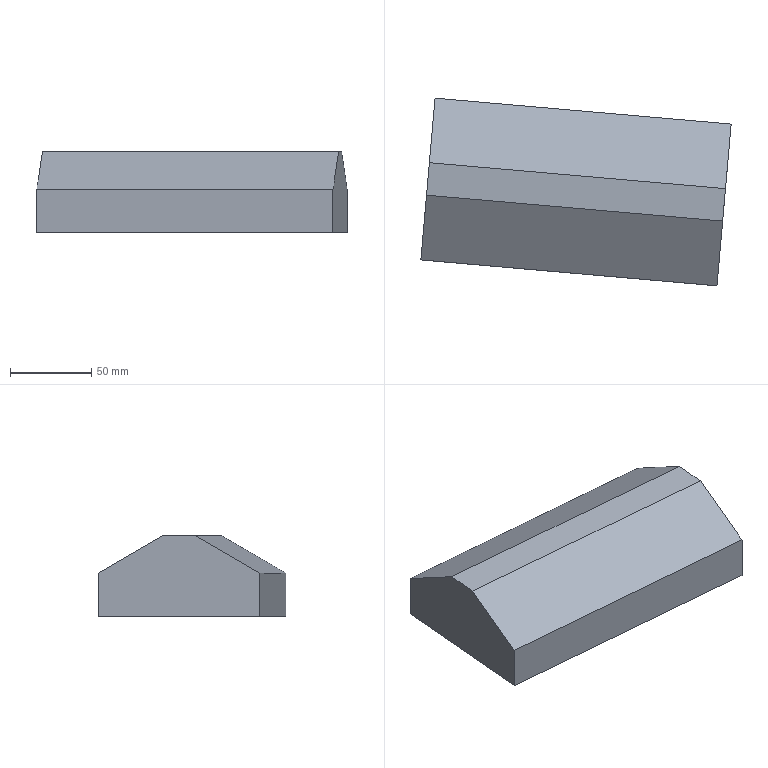Part | NX | features solid 2 | 1 solid | 8 faces | box 190.488 x 115.147 x 49.531 mm | volume 733523 mm3 | plane 8
STEP:
#1=CARTESIAN_POINT('',(-842.956,490.525,-243.453));
#2=VERTEX_POINT('',#1);
#3=CARTESIAN_POINT('',(-842.956,490.525,-270.));
#4=VERTEX_POINT('',#3);
#5=CARTESIAN_POINT('',(-842.956,490.525,-243.453));
#6=DIRECTION('',(0.,0.,-1.));
#7=VECTOR('',#6,1000.);
#8=LINE('',#5,#7);
#9=EDGE_CURVE('',#2,#4,#8,.T.);
#10=ORIENTED_EDGE('',*,*,#9,.F.);
#11=CARTESIAN_POINT('',(-1024.761,506.431,-243.453));
#12=VERTEX_POINT('',#11);
#13=CARTESIAN_POINT('',(-1024.761,506.431,-243.453));
#14=DIRECTION('',(0.9962,-0.08716,0.));
#15=VECTOR('',#14,1000.);
#16=LINE('',#13,#15);
#17=EDGE_CURVE('',#12,#2,#16,.T.);
#18=ORIENTED_EDGE('',*,*,#17,.F.);
#19=CARTESIAN_POINT('',(-1024.761,506.431,-270.));
#20=VERTEX_POINT('',#19);
#21=CARTESIAN_POINT('',(-1024.761,506.431,-243.453));
#22=DIRECTION('',(0.,0.,-1.));
#23=VECTOR('',#22,1000.);
#24=LINE('',#21,#23);
#25=EDGE_CURVE('',#12,#20,#24,.T.);
#26=ORIENTED_EDGE('',*,*,#25,.T.);
#27=CARTESIAN_POINT('',(-1024.761,506.431,-270.));
#28=DIRECTION('',(-0.9962,0.08716,0.));
#29=VECTOR('',#28,1000.);
#30=LINE('',#27,#29);
#31=EDGE_CURVE('',#20,#4,#30,.F.);
#32=ORIENTED_EDGE('',*,*,#31,.T.);
#33=EDGE_LOOP('',(#10,#18,#26,#32));
#34=FACE_BOUND('',#33,.T.);
#35=CARTESIAN_POINT('',(-1024.761,506.431,-243.453));
#36=DIRECTION('',(-0.08716,-0.9962,0.));
#37=DIRECTION('',(0.,0.,-1.));
#38=AXIS2_PLACEMENT_3D('',#35,#36,#37);
#39=PLANE('',#38);
#40=ADVANCED_FACE('',(#34),#39,.T.);
#41=CARTESIAN_POINT('',(-834.273,589.766,-270.));
#42=VERTEX_POINT('',#41);
#43=CARTESIAN_POINT('',(-842.956,490.525,-270.));
#44=DIRECTION('',(0.08716,0.9962,0.));
#45=VECTOR('',#44,1000.);
#46=LINE('',#43,#45);
#47=EDGE_CURVE('',#42,#4,#46,.F.);
#48=ORIENTED_EDGE('',*,*,#47,.T.);
#49=ORIENTED_EDGE('',*,*,#31,.F.);
#50=CARTESIAN_POINT('',(-1016.079,605.672,-270.));
#51=VERTEX_POINT('',#50);
#52=CARTESIAN_POINT('',(-1024.761,506.431,-270.));
#53=DIRECTION('',(0.08716,0.9962,0.));
#54=VECTOR('',#53,1000.);
#55=LINE('',#52,#54);
#56=EDGE_CURVE('',#51,#20,#55,.F.);
#57=ORIENTED_EDGE('',*,*,#56,.F.);
#58=CARTESIAN_POINT('',(-1016.079,605.672,-270.));
#59=DIRECTION('',(-0.9962,0.08716,0.));
#60=VECTOR('',#59,1000.);
#61=LINE('',#58,#60);
#62=EDGE_CURVE('',#51,#42,#61,.F.);
#63=ORIENTED_EDGE('',*,*,#62,.T.);
#64=EDGE_LOOP('',(#48,#49,#57,#63));
#65=FACE_BOUND('',#64,.T.);
#66=CARTESIAN_POINT('',(-1006.475,715.443,-270.));
#67=DIRECTION('',(0.,0.,-1.));
#68=DIRECTION('',(-0.9962,0.08716,0.));
#69=AXIS2_PLACEMENT_3D('',#66,#67,#68);
#70=PLANE('',#69);
#71=ADVANCED_FACE('',(#65),#70,.T.);
#72=CARTESIAN_POINT('',(-834.273,589.766,-243.453));
#73=VERTEX_POINT('',#72);
#74=CARTESIAN_POINT('',(-834.273,589.766,-243.453));
#75=DIRECTION('',(0.,0.,-1.));
#76=VECTOR('',#75,1000.);
#77=LINE('',#74,#76);
#78=EDGE_CURVE('',#73,#42,#77,.T.);
#79=ORIENTED_EDGE('',*,*,#78,.T.);
#80=ORIENTED_EDGE('',*,*,#62,.F.);
#81=CARTESIAN_POINT('',(-1016.079,605.672,-243.453));
#82=VERTEX_POINT('',#81);
#83=CARTESIAN_POINT('',(-1016.079,605.672,-243.453));
#84=DIRECTION('',(0.,0.,-1.));
#85=VECTOR('',#84,1000.);
#86=LINE('',#83,#85);
#87=EDGE_CURVE('',#82,#51,#86,.T.);
#88=ORIENTED_EDGE('',*,*,#87,.F.);
#89=CARTESIAN_POINT('',(-1016.079,605.672,-243.453));
#90=DIRECTION('',(0.9962,-0.08716,0.));
#91=VECTOR('',#90,1000.);
#92=LINE('',#89,#91);
#93=EDGE_CURVE('',#82,#73,#92,.T.);
#94=ORIENTED_EDGE('',*,*,#93,.T.);
#95=EDGE_LOOP('',(#79,#80,#88,#94));
#96=FACE_BOUND('',#95,.T.);
#97=CARTESIAN_POINT('',(-1016.079,605.672,-243.453));
#98=DIRECTION('',(-0.08716,-0.9962,0.));
#99=DIRECTION('',(0.,0.,-1.));
#100=AXIS2_PLACEMENT_3D('',#97,#98,#99);
#101=PLANE('',#100);
#102=ADVANCED_FACE('',(#96),#101,.F.);
#103=CARTESIAN_POINT('',(-837.743,550.107,-220.469));
#104=VERTEX_POINT('',#103);
#105=CARTESIAN_POINT('',(-837.743,550.107,-220.469));
#106=DIRECTION('',(0.07548,0.8627,-0.5));
#107=VECTOR('',#106,1000.);
#108=LINE('',#105,#107);
#109=EDGE_CURVE('',#104,#73,#108,.T.);
#110=ORIENTED_EDGE('',*,*,#109,.T.);
#111=ORIENTED_EDGE('',*,*,#93,.F.);
#112=CARTESIAN_POINT('',(-1019.548,566.013,-220.469));
#113=VERTEX_POINT('',#112);
#114=CARTESIAN_POINT('',(-1019.548,566.013,-220.469));
#115=DIRECTION('',(0.07548,0.8627,-0.5));
#116=VECTOR('',#115,1000.);
#117=LINE('',#114,#116);
#118=EDGE_CURVE('',#113,#82,#117,.T.);
#119=ORIENTED_EDGE('',*,*,#118,.F.);
#120=CARTESIAN_POINT('',(-1019.548,566.013,-220.469));
#121=DIRECTION('',(0.9962,-0.08716,0.));
#122=VECTOR('',#121,1000.);
#123=LINE('',#120,#122);
#124=EDGE_CURVE('',#113,#104,#123,.T.);
#125=ORIENTED_EDGE('',*,*,#124,.T.);
#126=EDGE_LOOP('',(#110,#111,#119,#125));
#127=FACE_BOUND('',#126,.T.);
#128=CARTESIAN_POINT('',(-1019.548,566.013,-220.469));
#129=DIRECTION('',(-0.04358,-0.4981,-0.866));
#130=DIRECTION('',(0.07548,0.8627,-0.5));
#131=AXIS2_PLACEMENT_3D('',#128,#129,#130);
#132=PLANE('',#131);
#133=ADVANCED_FACE('',(#127),#132,.F.);
#134=CARTESIAN_POINT('',(-839.486,530.184,-220.469));
#135=VERTEX_POINT('',#134);
#136=CARTESIAN_POINT('',(-839.486,530.184,-220.469));
#137=DIRECTION('',(0.08716,0.9962,0.));
#138=VECTOR('',#137,1000.);
#139=LINE('',#136,#138);
#140=EDGE_CURVE('',#135,#104,#139,.T.);
#141=ORIENTED_EDGE('',*,*,#140,.T.);
#142=ORIENTED_EDGE('',*,*,#124,.F.);
#143=CARTESIAN_POINT('',(-1021.291,546.089,-220.469));
#144=VERTEX_POINT('',#143);
#145=CARTESIAN_POINT('',(-1021.291,546.089,-220.469));
#146=DIRECTION('',(0.08716,0.9962,0.));
#147=VECTOR('',#146,1000.);
#148=LINE('',#145,#147);
#149=EDGE_CURVE('',#144,#113,#148,.T.);
#150=ORIENTED_EDGE('',*,*,#149,.F.);
#151=CARTESIAN_POINT('',(-1021.291,546.089,-220.469));
#152=DIRECTION('',(0.9962,-0.08716,0.));
#153=VECTOR('',#152,1000.);
#154=LINE('',#151,#153);
#155=EDGE_CURVE('',#144,#135,#154,.T.);
#156=ORIENTED_EDGE('',*,*,#155,.T.);
#157=EDGE_LOOP('',(#141,#142,#150,#156));
#158=FACE_BOUND('',#157,.T.);
#159=CARTESIAN_POINT('',(-1021.291,546.089,-220.469));
#160=DIRECTION('',(0.,0.,-1.));
#161=DIRECTION('',(0.08716,0.9962,0.));
#162=AXIS2_PLACEMENT_3D('',#159,#160,#161);
#163=PLANE('',#162);
#164=ADVANCED_FACE('',(#158),#163,.F.);
#165=CARTESIAN_POINT('',(-839.486,530.184,-220.469));
#166=DIRECTION('',(-0.07548,-0.8627,-0.5));
#167=VECTOR('',#166,1000.);
#168=LINE('',#165,#167);
#169=EDGE_CURVE('',#135,#2,#168,.T.);
#170=ORIENTED_EDGE('',*,*,#169,.F.);
#171=ORIENTED_EDGE('',*,*,#155,.F.);
#172=CARTESIAN_POINT('',(-1021.291,546.089,-220.469));
#173=DIRECTION('',(-0.07548,-0.8627,-0.5));
#174=VECTOR('',#173,1000.);
#175=LINE('',#172,#174);
#176=EDGE_CURVE('',#144,#12,#175,.T.);
#177=ORIENTED_EDGE('',*,*,#176,.T.);
#178=ORIENTED_EDGE('',*,*,#17,.T.);
#179=EDGE_LOOP('',(#170,#171,#177,#178));
#180=FACE_BOUND('',#179,.T.);
#181=CARTESIAN_POINT('',(-1021.291,546.089,-220.469));
#182=DIRECTION('',(-0.04358,-0.4981,0.866));
#183=DIRECTION('',(-0.07548,-0.8627,-0.5));
#184=AXIS2_PLACEMENT_3D('',#181,#182,#183);
#185=PLANE('',#184);
#186=ADVANCED_FACE('',(#180),#185,.T.);
#187=ORIENTED_EDGE('',*,*,#25,.F.);
#188=ORIENTED_EDGE('',*,*,#176,.F.);
#189=ORIENTED_EDGE('',*,*,#149,.T.);
#190=ORIENTED_EDGE('',*,*,#118,.T.);
#191=ORIENTED_EDGE('',*,*,#87,.T.);
#192=ORIENTED_EDGE('',*,*,#56,.T.);
#193=EDGE_LOOP('',(#187,#188,#189,#190,#191,#192));
#194=FACE_BOUND('',#193,.T.);
#195=CARTESIAN_POINT('',(-1024.761,506.431,-258.453));
#196=DIRECTION('',(0.9962,-0.08716,0.));
#197=DIRECTION('',(0.,0.,-1.));
#198=AXIS2_PLACEMENT_3D('',#195,#196,#197);
#199=PLANE('',#198);
#200=ADVANCED_FACE('',(#194),#199,.F.);
#201=ORIENTED_EDGE('',*,*,#9,.T.);
#202=ORIENTED_EDGE('',*,*,#47,.F.);
#203=ORIENTED_EDGE('',*,*,#78,.F.);
#204=ORIENTED_EDGE('',*,*,#109,.F.);
#205=ORIENTED_EDGE('',*,*,#140,.F.);
#206=ORIENTED_EDGE('',*,*,#169,.T.);
#207=EDGE_LOOP('',(#201,#202,#203,#204,#205,#206));
#208=FACE_BOUND('',#207,.T.);
#209=CARTESIAN_POINT('',(-842.956,490.525,-258.453));
#210=DIRECTION('',(0.9962,-0.08716,0.));
#211=DIRECTION('',(0.,0.,-1.));
#212=AXIS2_PLACEMENT_3D('',#209,#210,#211);
#213=PLANE('',#212);
#214=ADVANCED_FACE('',(#208),#213,.T.);
#215=CLOSED_SHELL('',(#40,#71,#102,#133,#164,#186,#200,#214));
#216=MANIFOLD_SOLID_BREP('',#215);
#217=(LENGTH_UNIT()NAMED_UNIT(*)SI_UNIT(.MILLI.,.METRE.));
#218=UNCERTAINTY_MEASURE_WITH_UNIT(LENGTH_MEASURE(0.00001),#217,'','');
#219=(NAMED_UNIT(*)PLANE_ANGLE_UNIT()SI_UNIT($,.RADIAN.));
#220=(NAMED_UNIT(*)SI_UNIT($,.STERADIAN.)SOLID_ANGLE_UNIT());
#221=(GEOMETRIC_REPRESENTATION_CONTEXT(3)GLOBAL_UNCERTAINTY_ASSIGNED_CONTEXT((#218))GLOBAL_UNIT_ASSIGNED_CONTEXT((#217,#219,#220))REPRESENTATION_CONTEXT('',''));
#222=ADVANCED_BREP_SHAPE_REPRESENTATION('',(#216),#221);